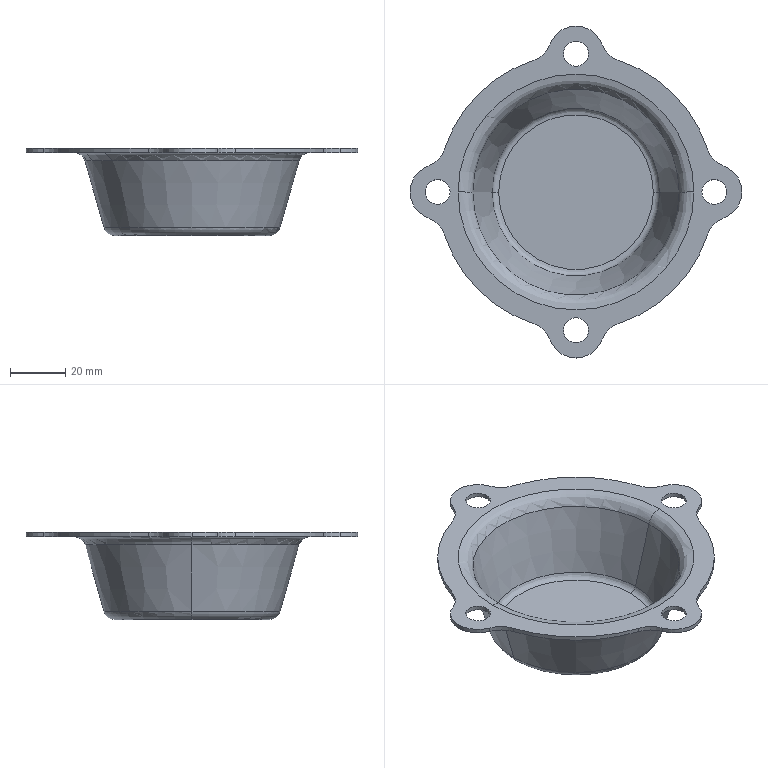Part | SolidWorks | features Boss 1, Extrusion 1, Fillet 1, RefAxis 1, Shell 1 | 1 solid | 41 faces | box 120 x 120 x 31.5 mm | volume 19269 mm3 | cylinder 25 | torus 8 | cone 4 | plane 4 | commonest cylinder face diameters 20 x13 9 x8 100 x4
STEP:
#1=CARTESIAN_POINT('',(42.584,0.,1.5));
#2=VERTEX_POINT('',#1);
#3=CARTESIAN_POINT('',(-42.584,0.,1.5));
#4=VERTEX_POINT('',#3);
#5=CARTESIAN_POINT('',(0.,0.,1.5));
#6=DIRECTION('',(0.,0.,1.));
#7=DIRECTION('',(1.,0.,0.));
#8=AXIS2_PLACEMENT_3D('',#5,#6,#7);
#9=CIRCLE('',#8,42.584);
#10=EDGE_CURVE('',#2,#4,#9,.T.);
#11=ORIENTED_EDGE('',*,*,#10,.T.);
#12=CARTESIAN_POINT('',(-37.297,0.,-2.484));
#13=VERTEX_POINT('',#12);
#14=CARTESIAN_POINT('',(-42.584,0.,-4.));
#15=DIRECTION('',(0.,1.,0.));
#16=DIRECTION('',(-1.,0.,0.));
#17=AXIS2_PLACEMENT_3D('',#14,#15,#16);
#18=CIRCLE('',#17,5.5);
#19=EDGE_CURVE('',#4,#13,#18,.T.);
#20=ORIENTED_EDGE('',*,*,#19,.T.);
#21=CARTESIAN_POINT('',(37.297,0.,-2.484));
#22=VERTEX_POINT('',#21);
#23=CARTESIAN_POINT('',(0.,0.,-2.484));
#24=DIRECTION('',(0.,0.,-1.));
#25=DIRECTION('',(1.,0.,0.));
#26=AXIS2_PLACEMENT_3D('',#23,#24,#25);
#27=CIRCLE('',#26,37.297);
#28=EDGE_CURVE('',#13,#22,#27,.T.);
#29=ORIENTED_EDGE('',*,*,#28,.T.);
#30=CARTESIAN_POINT('',(42.584,0.,-4.));
#31=DIRECTION('',(0.,-1.,0.));
#32=DIRECTION('',(0.,0.,-1.));
#33=AXIS2_PLACEMENT_3D('',#30,#31,#32);
#34=CIRCLE('',#33,5.5);
#35=EDGE_CURVE('',#2,#22,#34,.T.);
#36=ORIENTED_EDGE('',*,*,#35,.F.);
#37=EDGE_LOOP('',(#11,#20,#29,#36));
#38=FACE_OUTER_BOUND('',#37,.T.);
#39=CARTESIAN_POINT('',(0.,0.,-4.));
#40=DIRECTION('',(0.,0.,1.));
#41=DIRECTION('',(1.,0.,0.));
#42=AXIS2_PLACEMENT_3D('',#39,#40,#41);
#43=TOROIDAL_SURFACE('',#42,42.584,5.5);
#44=ADVANCED_FACE('',(#38),#43,.T.);
#45=CARTESIAN_POINT('',(27.953,0.,-28.5));
#46=VERTEX_POINT('',#45);
#47=CARTESIAN_POINT('',(-27.953,0.,-28.5));
#48=VERTEX_POINT('',#47);
#49=CARTESIAN_POINT('',(0.,0.,-28.5));
#50=DIRECTION('',(0.,0.,-1.));
#51=DIRECTION('',(1.,0.,0.));
#52=AXIS2_PLACEMENT_3D('',#49,#50,#51);
#53=CIRCLE('',#52,27.953);
#54=EDGE_CURVE('',#46,#48,#53,.T.);
#55=ORIENTED_EDGE('',*,*,#54,.T.);
#56=CARTESIAN_POINT('',(-30.356,0.,-26.689));
#57=VERTEX_POINT('',#56);
#58=CARTESIAN_POINT('',(-27.953,0.,-26.));
#59=DIRECTION('',(0.,1.,0.));
#60=DIRECTION('',(-1.,0.,0.));
#61=AXIS2_PLACEMENT_3D('',#58,#59,#60);
#62=CIRCLE('',#61,2.5);
#63=EDGE_CURVE('',#48,#57,#62,.T.);
#64=ORIENTED_EDGE('',*,*,#63,.T.);
#65=CARTESIAN_POINT('',(30.356,0.,-26.689));
#66=VERTEX_POINT('',#65);
#67=CARTESIAN_POINT('',(0.,0.,-26.689));
#68=DIRECTION('',(0.,0.,1.));
#69=DIRECTION('',(1.,0.,0.));
#70=AXIS2_PLACEMENT_3D('',#67,#68,#69);
#71=CIRCLE('',#70,30.356);
#72=EDGE_CURVE('',#57,#66,#71,.T.);
#73=ORIENTED_EDGE('',*,*,#72,.T.);
#74=CARTESIAN_POINT('',(27.953,0.,-26.));
#75=DIRECTION('',(0.,-1.,0.));
#76=DIRECTION('',(0.,0.,-1.));
#77=AXIS2_PLACEMENT_3D('',#74,#75,#76);
#78=CIRCLE('',#77,2.5);
#79=EDGE_CURVE('',#46,#66,#78,.T.);
#80=ORIENTED_EDGE('',*,*,#79,.F.);
#81=EDGE_LOOP('',(#55,#64,#73,#80));
#82=FACE_OUTER_BOUND('',#81,.T.);
#83=CARTESIAN_POINT('',(0.,0.,-26.));
#84=DIRECTION('',(0.,0.,1.));
#85=DIRECTION('',(1.,0.,0.));
#86=AXIS2_PLACEMENT_3D('',#83,#84,#85);
#87=TOROIDAL_SURFACE('',#86,27.953,2.5);
#88=ADVANCED_FACE('',(#82),#87,.F.);
#89=ORIENTED_EDGE('',*,*,#72,.F.);
#90=CARTESIAN_POINT('',(-38.558,0.,1.913));
#91=DIRECTION('',(-0.2756,0.,0.9613));
#92=VECTOR('',#91,1000.);
#93=LINE('',#90,#92);
#94=EDGE_CURVE('',#57,#13,#93,.T.);
#95=ORIENTED_EDGE('',*,*,#94,.T.);
#96=CARTESIAN_POINT('',(0.,0.,-2.484));
#97=DIRECTION('',(0.,0.,-1.));
#98=DIRECTION('',(1.,0.,0.));
#99=AXIS2_PLACEMENT_3D('',#96,#97,#98);
#100=CIRCLE('',#99,37.297);
#101=EDGE_CURVE('',#22,#13,#100,.T.);
#102=ORIENTED_EDGE('',*,*,#101,.F.);
#103=CARTESIAN_POINT('',(38.558,0.,1.913));
#104=DIRECTION('',(0.2756,0.,0.9613));
#105=VECTOR('',#104,1000.);
#106=LINE('',#103,#105);
#107=EDGE_CURVE('',#66,#22,#106,.T.);
#108=ORIENTED_EDGE('',*,*,#107,.F.);
#109=EDGE_LOOP('',(#89,#95,#102,#108));
#110=FACE_OUTER_BOUND('',#109,.T.);
#111=CARTESIAN_POINT('',(0.,0.,1.913));
#112=DIRECTION('',(0.,0.,1.));
#113=DIRECTION('',(1.,0.,0.));
#114=AXIS2_PLACEMENT_3D('',#111,#112,#113);
#115=CONICAL_SURFACE('',#114,38.558,0.2793);
#116=ADVANCED_FACE('',(#110),#115,.F.);
#117=CARTESIAN_POINT('',(-42.584,0.,0.));
#118=VERTEX_POINT('',#117);
#119=CARTESIAN_POINT('',(42.584,0.,0.));
#120=VERTEX_POINT('',#119);
#121=CARTESIAN_POINT('',(0.,0.,0.));
#122=DIRECTION('',(0.,0.,1.));
#123=DIRECTION('',(1.,0.,0.));
#124=AXIS2_PLACEMENT_3D('',#121,#122,#123);
#125=CIRCLE('',#124,42.584);
#126=EDGE_CURVE('',#118,#120,#125,.T.);
#127=ORIENTED_EDGE('',*,*,#126,.F.);
#128=CARTESIAN_POINT('',(-38.739,0.,-2.897));
#129=VERTEX_POINT('',#128);
#130=CARTESIAN_POINT('',(-42.584,0.,-4.));
#131=DIRECTION('',(0.,1.,0.));
#132=DIRECTION('',(-1.,0.,0.));
#133=AXIS2_PLACEMENT_3D('',#130,#131,#132);
#134=CIRCLE('',#133,4.);
#135=EDGE_CURVE('',#118,#129,#134,.T.);
#136=ORIENTED_EDGE('',*,*,#135,.T.);
#137=CARTESIAN_POINT('',(38.739,0.,-2.897));
#138=VERTEX_POINT('',#137);
#139=CARTESIAN_POINT('',(0.,0.,-2.897));
#140=DIRECTION('',(0.,0.,-1.));
#141=DIRECTION('',(-1.,0.,0.));
#142=AXIS2_PLACEMENT_3D('',#139,#140,#141);
#143=CIRCLE('',#142,38.739);
#144=EDGE_CURVE('',#138,#129,#143,.T.);
#145=ORIENTED_EDGE('',*,*,#144,.F.);
#146=CARTESIAN_POINT('',(42.584,0.,-4.));
#147=DIRECTION('',(0.,-1.,0.));
#148=DIRECTION('',(0.,0.,-1.));
#149=AXIS2_PLACEMENT_3D('',#146,#147,#148);
#150=CIRCLE('',#149,4.);
#151=EDGE_CURVE('',#120,#138,#150,.T.);
#152=ORIENTED_EDGE('',*,*,#151,.F.);
#153=EDGE_LOOP('',(#127,#136,#145,#152));
#154=FACE_OUTER_BOUND('',#153,.T.);
#155=CARTESIAN_POINT('',(0.,0.,-4.));
#156=DIRECTION('',(0.,0.,1.));
#157=DIRECTION('',(1.,0.,0.));
#158=AXIS2_PLACEMENT_3D('',#155,#156,#157);
#159=TOROIDAL_SURFACE('',#158,42.584,4.);
#160=ADVANCED_FACE('',(#154),#159,.F.);
#161=CARTESIAN_POINT('',(-27.953,0.,-30.));
#162=VERTEX_POINT('',#161);
#163=CARTESIAN_POINT('',(27.953,0.,-30.));
#164=VERTEX_POINT('',#163);
#165=CARTESIAN_POINT('',(0.,0.,-30.));
#166=DIRECTION('',(0.,0.,-1.));
#167=DIRECTION('',(1.,0.,0.));
#168=AXIS2_PLACEMENT_3D('',#165,#166,#167);
#169=CIRCLE('',#168,27.953);
#170=EDGE_CURVE('',#162,#164,#169,.T.);
#171=ORIENTED_EDGE('',*,*,#170,.F.);
#172=CARTESIAN_POINT('',(-31.798,0.,-27.103));
#173=VERTEX_POINT('',#172);
#174=CARTESIAN_POINT('',(-27.953,0.,-26.));
#175=DIRECTION('',(0.,1.,0.));
#176=DIRECTION('',(-1.,0.,0.));
#177=AXIS2_PLACEMENT_3D('',#174,#175,#176);
#178=CIRCLE('',#177,4.);
#179=EDGE_CURVE('',#162,#173,#178,.T.);
#180=ORIENTED_EDGE('',*,*,#179,.T.);
#181=CARTESIAN_POINT('',(31.798,0.,-27.103));
#182=VERTEX_POINT('',#181);
#183=CARTESIAN_POINT('',(0.,0.,-27.103));
#184=DIRECTION('',(0.,0.,1.));
#185=DIRECTION('',(1.,0.,0.));
#186=AXIS2_PLACEMENT_3D('',#183,#184,#185);
#187=CIRCLE('',#186,31.798);
#188=EDGE_CURVE('',#182,#173,#187,.T.);
#189=ORIENTED_EDGE('',*,*,#188,.F.);
#190=CARTESIAN_POINT('',(27.953,0.,-26.));
#191=DIRECTION('',(0.,-1.,0.));
#192=DIRECTION('',(0.,0.,-1.));
#193=AXIS2_PLACEMENT_3D('',#190,#191,#192);
#194=CIRCLE('',#193,4.);
#195=EDGE_CURVE('',#164,#182,#194,.T.);
#196=ORIENTED_EDGE('',*,*,#195,.F.);
#197=EDGE_LOOP('',(#171,#180,#189,#196));
#198=FACE_OUTER_BOUND('',#197,.T.);
#199=CARTESIAN_POINT('',(0.,0.,-26.));
#200=DIRECTION('',(0.,0.,1.));
#201=DIRECTION('',(1.,0.,0.));
#202=AXIS2_PLACEMENT_3D('',#199,#200,#201);
#203=TOROIDAL_SURFACE('',#202,27.953,4.);
#204=ADVANCED_FACE('',(#198),#203,.T.);
#205=ORIENTED_EDGE('',*,*,#188,.T.);
#206=CARTESIAN_POINT('',(-40.,0.,1.5));
#207=DIRECTION('',(-0.2756,0.,0.9613));
#208=VECTOR('',#207,1000.);
#209=LINE('',#206,#208);
#210=EDGE_CURVE('',#173,#129,#209,.T.);
#211=ORIENTED_EDGE('',*,*,#210,.T.);
#212=CARTESIAN_POINT('',(0.,0.,-2.897));
#213=DIRECTION('',(0.,0.,-1.));
#214=DIRECTION('',(-1.,0.,0.));
#215=AXIS2_PLACEMENT_3D('',#212,#213,#214);
#216=CIRCLE('',#215,38.739);
#217=EDGE_CURVE('',#129,#138,#216,.T.);
#218=ORIENTED_EDGE('',*,*,#217,.T.);
#219=CARTESIAN_POINT('',(40.,0.,1.5));
#220=DIRECTION('',(0.2756,0.,0.9613));
#221=VECTOR('',#220,1000.);
#222=LINE('',#219,#221);
#223=EDGE_CURVE('',#182,#138,#222,.T.);
#224=ORIENTED_EDGE('',*,*,#223,.F.);
#225=EDGE_LOOP('',(#205,#211,#218,#224));
#226=FACE_OUTER_BOUND('',#225,.T.);
#227=CARTESIAN_POINT('',(0.,0.,1.5));
#228=DIRECTION('',(0.,0.,1.));
#229=DIRECTION('',(1.,0.,0.));
#230=AXIS2_PLACEMENT_3D('',#227,#228,#229);
#231=CONICAL_SURFACE('',#230,40.,0.2793);
#232=ADVANCED_FACE('',(#226),#231,.T.);
#233=CARTESIAN_POINT('',(45.5,0.,1.5));
#234=VERTEX_POINT('',#233);
#235=CARTESIAN_POINT('',(54.5,0.,1.5));
#236=VERTEX_POINT('',#235);
#237=CARTESIAN_POINT('',(50.,0.,1.5));
#238=DIRECTION('',(0.,0.,1.));
#239=DIRECTION('',(1.,0.,0.));
#240=AXIS2_PLACEMENT_3D('',#237,#238,#239);
#241=CIRCLE('',#240,4.5);
#242=EDGE_CURVE('',#234,#236,#241,.T.);
#243=ORIENTED_EDGE('',*,*,#242,.T.);
#244=CARTESIAN_POINT('',(54.5,0.,0.));
#245=VERTEX_POINT('',#244);
#246=CARTESIAN_POINT('',(54.5,0.,1.5));
#247=DIRECTION('',(0.,0.,-1.));
#248=VECTOR('',#247,1000.);
#249=LINE('',#246,#248);
#250=EDGE_CURVE('',#236,#245,#249,.T.);
#251=ORIENTED_EDGE('',*,*,#250,.T.);
#252=CARTESIAN_POINT('',(45.5,0.,0.));
#253=VERTEX_POINT('',#252);
#254=CARTESIAN_POINT('',(50.,0.,0.));
#255=DIRECTION('',(0.,0.,1.));
#256=DIRECTION('',(1.,0.,0.));
#257=AXIS2_PLACEMENT_3D('',#254,#255,#256);
#258=CIRCLE('',#257,4.5);
#259=EDGE_CURVE('',#253,#245,#258,.T.);
#260=ORIENTED_EDGE('',*,*,#259,.F.);
#261=CARTESIAN_POINT('',(45.5,0.,1.5));
#262=DIRECTION('',(0.,0.,-1.));
#263=VECTOR('',#262,1000.);
#264=LINE('',#261,#263);
#265=EDGE_CURVE('',#234,#253,#264,.T.);
#266=ORIENTED_EDGE('',*,*,#265,.F.);
#267=EDGE_LOOP('',(#243,#251,#260,#266));
#268=FACE_OUTER_BOUND('',#267,.T.);
#269=CARTESIAN_POINT('',(50.,0.,1.5));
#270=DIRECTION('',(0.,0.,-1.));
#271=DIRECTION('',(-1.,0.,0.));
#272=AXIS2_PLACEMENT_3D('',#269,#270,#271);
#273=CYLINDRICAL_SURFACE('',#272,4.5);
#274=ADVANCED_FACE('',(#268),#273,.F.);
#275=CARTESIAN_POINT('',(-4.5,-50.,1.5));
#276=VERTEX_POINT('',#275);
#277=CARTESIAN_POINT('',(4.5,-50.,1.5));
#278=VERTEX_POINT('',#277);
#279=CARTESIAN_POINT('',(0.,-50.,1.5));
#280=DIRECTION('',(0.,0.,1.));
#281=DIRECTION('',(1.,0.,0.));
#282=AXIS2_PLACEMENT_3D('',#279,#280,#281);
#283=CIRCLE('',#282,4.5);
#284=EDGE_CURVE('',#276,#278,#283,.T.);
#285=ORIENTED_EDGE('',*,*,#284,.T.);
#286=CARTESIAN_POINT('',(4.5,-50.,0.));
#287=VERTEX_POINT('',#286);
#288=CARTESIAN_POINT('',(4.5,-50.,1.5));
#289=DIRECTION('',(0.,0.,-1.));
#290=VECTOR('',#289,1000.);
#291=LINE('',#288,#290);
#292=EDGE_CURVE('',#278,#287,#291,.T.);
#293=ORIENTED_EDGE('',*,*,#292,.T.);
#294=CARTESIAN_POINT('',(-4.5,-50.,0.));
#295=VERTEX_POINT('',#294);
#296=CARTESIAN_POINT('',(0.,-50.,0.));
#297=DIRECTION('',(0.,0.,1.));
#298=DIRECTION('',(1.,0.,0.));
#299=AXIS2_PLACEMENT_3D('',#296,#297,#298);
#300=CIRCLE('',#299,4.5);
#301=EDGE_CURVE('',#295,#287,#300,.T.);
#302=ORIENTED_EDGE('',*,*,#301,.F.);
#303=CARTESIAN_POINT('',(-4.5,-50.,1.5));
#304=DIRECTION('',(0.,0.,-1.));
#305=VECTOR('',#304,1000.);
#306=LINE('',#303,#305);
#307=EDGE_CURVE('',#276,#295,#306,.T.);
#308=ORIENTED_EDGE('',*,*,#307,.F.);
#309=EDGE_LOOP('',(#285,#293,#302,#308));
#310=FACE_OUTER_BOUND('',#309,.T.);
#311=CARTESIAN_POINT('',(0.,-50.,1.5));
#312=DIRECTION('',(0.,0.,-1.));
#313=DIRECTION('',(-1.,0.,0.));
#314=AXIS2_PLACEMENT_3D('',#311,#312,#313);
#315=CYLINDRICAL_SURFACE('',#314,4.5);
#316=ADVANCED_FACE('',(#310),#315,.F.);
#317=CARTESIAN_POINT('',(-54.5,0.,1.5));
#318=VERTEX_POINT('',#317);
#319=CARTESIAN_POINT('',(-45.5,0.,1.5));
#320=VERTEX_POINT('',#319);
#321=CARTESIAN_POINT('',(-50.,0.,1.5));
#322=DIRECTION('',(0.,0.,1.));
#323=DIRECTION('',(1.,0.,0.));
#324=AXIS2_PLACEMENT_3D('',#321,#322,#323);
#325=CIRCLE('',#324,4.5);
#326=EDGE_CURVE('',#318,#320,#325,.T.);
#327=ORIENTED_EDGE('',*,*,#326,.T.);
#328=CARTESIAN_POINT('',(-45.5,0.,0.));
#329=VERTEX_POINT('',#328);
#330=CARTESIAN_POINT('',(-45.5,0.,1.5));
#331=DIRECTION('',(0.,0.,-1.));
#332=VECTOR('',#331,1000.);
#333=LINE('',#330,#332);
#334=EDGE_CURVE('',#320,#329,#333,.T.);
#335=ORIENTED_EDGE('',*,*,#334,.T.);
#336=CARTESIAN_POINT('',(-54.5,0.,0.));
#337=VERTEX_POINT('',#336);
#338=CARTESIAN_POINT('',(-50.,0.,0.));
#339=DIRECTION('',(0.,0.,1.));
#340=DIRECTION('',(1.,0.,0.));
#341=AXIS2_PLACEMENT_3D('',#338,#339,#340);
#342=CIRCLE('',#341,4.5);
#343=EDGE_CURVE('',#337,#329,#342,.T.);
#344=ORIENTED_EDGE('',*,*,#343,.F.);
#345=CARTESIAN_POINT('',(-54.5,0.,1.5));
#346=DIRECTION('',(0.,0.,-1.));
#347=VECTOR('',#346,1000.);
#348=LINE('',#345,#347);
#349=EDGE_CURVE('',#318,#337,#348,.T.);
#350=ORIENTED_EDGE('',*,*,#349,.F.);
#351=EDGE_LOOP('',(#327,#335,#344,#350));
#352=FACE_OUTER_BOUND('',#351,.T.);
#353=CARTESIAN_POINT('',(-50.,0.,1.5));
#354=DIRECTION('',(0.,0.,-1.));
#355=DIRECTION('',(-1.,0.,0.));
#356=AXIS2_PLACEMENT_3D('',#353,#354,#355);
#357=CYLINDRICAL_SURFACE('',#356,4.5);
#358=ADVANCED_FACE('',(#352),#357,.F.);
#359=CARTESIAN_POINT('',(-4.5,50.,1.5));
#360=VERTEX_POINT('',#359);
#361=CARTESIAN_POINT('',(4.5,50.,1.5));
#362=VERTEX_POINT('',#361);
#363=CARTESIAN_POINT('',(0.,50.,1.5));
#364=DIRECTION('',(0.,0.,1.));
#365=DIRECTION('',(1.,0.,0.));
#366=AXIS2_PLACEMENT_3D('',#363,#364,#365);
#367=CIRCLE('',#366,4.5);
#368=EDGE_CURVE('',#360,#362,#367,.T.);
#369=ORIENTED_EDGE('',*,*,#368,.T.);
#370=CARTESIAN_POINT('',(4.5,50.,0.));
#371=VERTEX_POINT('',#370);
#372=CARTESIAN_POINT('',(4.5,50.,1.5));
#373=DIRECTION('',(0.,0.,-1.));
#374=VECTOR('',#373,1000.);
#375=LINE('',#372,#374);
#376=EDGE_CURVE('',#362,#371,#375,.T.);
#377=ORIENTED_EDGE('',*,*,#376,.T.);
#378=CARTESIAN_POINT('',(-4.5,50.,0.));
#379=VERTEX_POINT('',#378);
#380=CARTESIAN_POINT('',(0.,50.,0.));
#381=DIRECTION('',(0.,0.,1.));
#382=DIRECTION('',(1.,0.,0.));
#383=AXIS2_PLACEMENT_3D('',#380,#381,#382);
#384=CIRCLE('',#383,4.5);
#385=EDGE_CURVE('',#379,#371,#384,.T.);
#386=ORIENTED_EDGE('',*,*,#385,.F.);
#387=CARTESIAN_POINT('',(-4.5,50.,1.5));
#388=DIRECTION('',(0.,0.,-1.));
#389=VECTOR('',#388,1000.);
#390=LINE('',#387,#389);
#391=EDGE_CURVE('',#360,#379,#390,.T.);
#392=ORIENTED_EDGE('',*,*,#391,.F.);
#393=EDGE_LOOP('',(#369,#377,#386,#392));
#394=FACE_OUTER_BOUND('',#393,.T.);
#395=CARTESIAN_POINT('',(0.,50.,1.5));
#396=DIRECTION('',(0.,0.,-1.));
#397=DIRECTION('',(-1.,0.,0.));
#398=AXIS2_PLACEMENT_3D('',#395,#396,#397);
#399=CYLINDRICAL_SURFACE('',#398,4.5);
#400=ADVANCED_FACE('',(#394),#399,.F.);
#401=CARTESIAN_POINT('',(-60.,0.,1.5));
#402=VERTEX_POINT('',#401);
#403=CARTESIAN_POINT('',(-53.5,-9.367,1.5));
#404=VERTEX_POINT('',#403);
#405=CARTESIAN_POINT('',(-50.,0.,1.5));
#406=DIRECTION('',(0.,0.,1.));
#407=DIRECTION('',(1.,0.,0.));
#408=AXIS2_PLACEMENT_3D('',#405,#406,#407);
#409=CIRCLE('',#408,10.);
#410=EDGE_CURVE('',#402,#404,#409,.T.);
#411=ORIENTED_EDGE('',*,*,#410,.F.);
#412=CARTESIAN_POINT('',(-60.,0.,0.));
#413=VERTEX_POINT('',#412);
#414=CARTESIAN_POINT('',(-60.,0.,1.5));
#415=DIRECTION('',(0.,0.,-1.));
#416=VECTOR('',#415,1000.);
#417=LINE('',#414,#416);
#418=EDGE_CURVE('',#402,#413,#417,.T.);
#419=ORIENTED_EDGE('',*,*,#418,.T.);
#420=CARTESIAN_POINT('',(-53.5,-9.367,0.));
#421=VERTEX_POINT('',#420);
#422=CARTESIAN_POINT('',(-50.,0.,0.));
#423=DIRECTION('',(0.,0.,1.));
#424=DIRECTION('',(1.,0.,0.));
#425=AXIS2_PLACEMENT_3D('',#422,#423,#424);
#426=CIRCLE('',#425,10.);
#427=EDGE_CURVE('',#413,#421,#426,.T.);
#428=ORIENTED_EDGE('',*,*,#427,.T.);
#429=CARTESIAN_POINT('',(-53.5,-9.367,1.5));
#430=DIRECTION('',(0.,0.,-1.));
#431=VECTOR('',#430,1000.);
#432=LINE('',#429,#431);
#433=EDGE_CURVE('',#404,#421,#432,.T.);
#434=ORIENTED_EDGE('',*,*,#433,.F.);
#435=EDGE_LOOP('',(#411,#419,#428,#434));
#436=FACE_OUTER_BOUND('',#435,.T.);
#437=CARTESIAN_POINT('',(-50.,0.,1.5));
#438=DIRECTION('',(0.,0.,-1.));
#439=DIRECTION('',(-1.,0.,0.));
#440=AXIS2_PLACEMENT_3D('',#437,#438,#439);
#441=CYLINDRICAL_SURFACE('',#440,10.);
#442=ADVANCED_FACE('',(#436),#441,.T.);
#443=ORIENTED_EDGE('',*,*,#10,.F.);
#444=CARTESIAN_POINT('',(0.,0.,1.5));
#445=DIRECTION('',(0.,0.,1.));
#446=DIRECTION('',(1.,0.,0.));
#447=AXIS2_PLACEMENT_3D('',#444,#445,#446);
#448=CIRCLE('',#447,42.584);
#449=EDGE_CURVE('',#4,#2,#448,.T.);
#450=ORIENTED_EDGE('',*,*,#449,.F.);
#451=EDGE_LOOP('',(#443,#450));
#452=FACE_BOUND('',#451,.T.);
#453=ORIENTED_EDGE('',*,*,#284,.F.);
#454=CARTESIAN_POINT('',(0.,-50.,1.5));
#455=DIRECTION('',(0.,0.,1.));
#456=DIRECTION('',(1.,0.,0.));
#457=AXIS2_PLACEMENT_3D('',#454,#455,#456);
#458=CIRCLE('',#457,4.5);
#459=EDGE_CURVE('',#278,#276,#458,.T.);
#460=ORIENTED_EDGE('',*,*,#459,.F.);
#461=EDGE_LOOP('',(#453,#460));
#462=FACE_BOUND('',#461,.T.);
#463=ORIENTED_EDGE('',*,*,#368,.F.);
#464=CARTESIAN_POINT('',(0.,50.,1.5));
#465=DIRECTION('',(0.,0.,1.));
#466=DIRECTION('',(1.,0.,0.));
#467=AXIS2_PLACEMENT_3D('',#464,#465,#466);
#468=CIRCLE('',#467,4.5);
#469=EDGE_CURVE('',#362,#360,#468,.T.);
#470=ORIENTED_EDGE('',*,*,#469,.F.);
#471=EDGE_LOOP('',(#463,#470));
#472=FACE_BOUND('',#471,.T.);
#473=CARTESIAN_POINT('',(-9.367,53.5,1.5));
#474=VERTEX_POINT('',#473);
#475=CARTESIAN_POINT('',(-15.612,47.5,1.5));
#476=VERTEX_POINT('',#475);
#477=CARTESIAN_POINT('',(-18.735,57.,1.5));
#478=DIRECTION('',(0.,0.,-1.));
#479=DIRECTION('',(1.,0.,0.));
#480=AXIS2_PLACEMENT_3D('',#477,#478,#479);
#481=CIRCLE('',#480,10.);
#482=EDGE_CURVE('',#474,#476,#481,.T.);
#483=ORIENTED_EDGE('',*,*,#482,.T.);
#484=CARTESIAN_POINT('',(-47.5,15.612,1.5));
#485=VERTEX_POINT('',#484);
#486=CARTESIAN_POINT('',(0.,0.,1.5));
#487=DIRECTION('',(0.,0.,1.));
#488=DIRECTION('',(1.,0.,0.));
#489=AXIS2_PLACEMENT_3D('',#486,#487,#488);
#490=CIRCLE('',#489,50.);
#491=EDGE_CURVE('',#476,#485,#490,.T.);
#492=ORIENTED_EDGE('',*,*,#491,.T.);
#493=CARTESIAN_POINT('',(-53.5,9.367,1.5));
#494=VERTEX_POINT('',#493);
#495=CARTESIAN_POINT('',(-57.,18.735,1.5));
#496=DIRECTION('',(0.,0.,-1.));
#497=DIRECTION('',(-1.,0.,0.));
#498=AXIS2_PLACEMENT_3D('',#495,#496,#497);
#499=CIRCLE('',#498,10.);
#500=EDGE_CURVE('',#485,#494,#499,.T.);
#501=ORIENTED_EDGE('',*,*,#500,.T.);
#502=CARTESIAN_POINT('',(-50.,0.,1.5));
#503=DIRECTION('',(0.,0.,1.));
#504=DIRECTION('',(1.,0.,0.));
#505=AXIS2_PLACEMENT_3D('',#502,#503,#504);
#506=CIRCLE('',#505,10.);
#507=EDGE_CURVE('',#494,#402,#506,.T.);
#508=ORIENTED_EDGE('',*,*,#507,.T.);
#509=ORIENTED_EDGE('',*,*,#410,.T.);
#510=CARTESIAN_POINT('',(-47.5,-15.612,1.5));
#511=VERTEX_POINT('',#510);
#512=CARTESIAN_POINT('',(-57.,-18.735,1.5));
#513=DIRECTION('',(0.,0.,-1.));
#514=DIRECTION('',(-1.,0.,0.));
#515=AXIS2_PLACEMENT_3D('',#512,#513,#514);
#516=CIRCLE('',#515,10.);
#517=EDGE_CURVE('',#404,#511,#516,.T.);
#518=ORIENTED_EDGE('',*,*,#517,.T.);
#519=CARTESIAN_POINT('',(-15.612,-47.5,1.5));
#520=VERTEX_POINT('',#519);
#521=CARTESIAN_POINT('',(0.,0.,1.5));
#522=DIRECTION('',(0.,0.,1.));
#523=DIRECTION('',(1.,0.,0.));
#524=AXIS2_PLACEMENT_3D('',#521,#522,#523);
#525=CIRCLE('',#524,50.);
#526=EDGE_CURVE('',#511,#520,#525,.T.);
#527=ORIENTED_EDGE('',*,*,#526,.T.);
#528=CARTESIAN_POINT('',(-9.367,-53.5,1.5));
#529=VERTEX_POINT('',#528);
#530=CARTESIAN_POINT('',(-18.735,-57.,1.5));
#531=DIRECTION('',(0.,0.,-1.));
#532=DIRECTION('',(-1.,0.,0.));
#533=AXIS2_PLACEMENT_3D('',#530,#531,#532);
#534=CIRCLE('',#533,10.);
#535=EDGE_CURVE('',#520,#529,#534,.T.);
#536=ORIENTED_EDGE('',*,*,#535,.T.);
#537=CARTESIAN_POINT('',(9.367,-53.5,1.5));
#538=VERTEX_POINT('',#537);
#539=CARTESIAN_POINT('',(0.,-50.,1.5));
#540=DIRECTION('',(0.,0.,1.));
#541=DIRECTION('',(1.,0.,0.));
#542=AXIS2_PLACEMENT_3D('',#539,#540,#541);
#543=CIRCLE('',#542,10.);
#544=EDGE_CURVE('',#529,#538,#543,.T.);
#545=ORIENTED_EDGE('',*,*,#544,.T.);
#546=CARTESIAN_POINT('',(15.612,-47.5,1.5));
#547=VERTEX_POINT('',#546);
#548=CARTESIAN_POINT('',(18.735,-57.,1.5));
#549=DIRECTION('',(0.,0.,-1.));
#550=DIRECTION('',(-1.,0.,0.));
#551=AXIS2_PLACEMENT_3D('',#548,#549,#550);
#552=CIRCLE('',#551,10.);
#553=EDGE_CURVE('',#538,#547,#552,.T.);
#554=ORIENTED_EDGE('',*,*,#553,.T.);
#555=CARTESIAN_POINT('',(47.5,-15.612,1.5));
#556=VERTEX_POINT('',#555);
#557=CARTESIAN_POINT('',(0.,0.,1.5));
#558=DIRECTION('',(0.,0.,1.));
#559=DIRECTION('',(1.,0.,0.));
#560=AXIS2_PLACEMENT_3D('',#557,#558,#559);
#561=CIRCLE('',#560,50.);
#562=EDGE_CURVE('',#547,#556,#561,.T.);
#563=ORIENTED_EDGE('',*,*,#562,.T.);
#564=CARTESIAN_POINT('',(53.5,-9.367,1.5));
#565=VERTEX_POINT('',#564);
#566=CARTESIAN_POINT('',(57.,-18.735,1.5));
#567=DIRECTION('',(0.,0.,-1.));
#568=DIRECTION('',(-1.,0.,0.));
#569=AXIS2_PLACEMENT_3D('',#566,#567,#568);
#570=CIRCLE('',#569,10.);
#571=EDGE_CURVE('',#556,#565,#570,.T.);
#572=ORIENTED_EDGE('',*,*,#571,.T.);
#573=CARTESIAN_POINT('',(53.5,9.367,1.5));
#574=VERTEX_POINT('',#573);
#575=CARTESIAN_POINT('',(50.,0.,1.5));
#576=DIRECTION('',(0.,0.,1.));
#577=DIRECTION('',(1.,0.,0.));
#578=AXIS2_PLACEMENT_3D('',#575,#576,#577);
#579=CIRCLE('',#578,10.);
#580=EDGE_CURVE('',#565,#574,#579,.T.);
#581=ORIENTED_EDGE('',*,*,#580,.T.);
#582=CARTESIAN_POINT('',(47.5,15.612,1.5));
#583=VERTEX_POINT('',#582);
#584=CARTESIAN_POINT('',(57.,18.735,1.5));
#585=DIRECTION('',(0.,0.,-1.));
#586=DIRECTION('',(-1.,0.,0.));
#587=AXIS2_PLACEMENT_3D('',#584,#585,#586);
#588=CIRCLE('',#587,10.);
#589=EDGE_CURVE('',#574,#583,#588,.T.);
#590=ORIENTED_EDGE('',*,*,#589,.T.);
#591=CARTESIAN_POINT('',(15.612,47.5,1.5));
#592=VERTEX_POINT('',#591);
#593=CARTESIAN_POINT('',(0.,0.,1.5));
#594=DIRECTION('',(0.,0.,1.));
#595=DIRECTION('',(1.,0.,0.));
#596=AXIS2_PLACEMENT_3D('',#593,#594,#595);
#597=CIRCLE('',#596,50.);
#598=EDGE_CURVE('',#583,#592,#597,.T.);
#599=ORIENTED_EDGE('',*,*,#598,.T.);
#600=CARTESIAN_POINT('',(9.367,53.5,1.5));
#601=VERTEX_POINT('',#600);
#602=CARTESIAN_POINT('',(18.735,57.,1.5));
#603=DIRECTION('',(0.,0.,-1.));
#604=DIRECTION('',(-1.,0.,0.));
#605=AXIS2_PLACEMENT_3D('',#602,#603,#604);
#606=CIRCLE('',#605,10.);
#607=EDGE_CURVE('',#592,#601,#606,.T.);
#608=ORIENTED_EDGE('',*,*,#607,.T.);
#609=CARTESIAN_POINT('',(0.,50.,1.5));
#610=DIRECTION('',(0.,0.,1.));
#611=DIRECTION('',(1.,0.,0.));
#612=AXIS2_PLACEMENT_3D('',#609,#610,#611);
#613=CIRCLE('',#612,10.);
#614=EDGE_CURVE('',#601,#474,#613,.T.);
#615=ORIENTED_EDGE('',*,*,#614,.T.);
#616=EDGE_LOOP('',(#483,#492,#501,#508,#509,#518,#527,#536,#545,#554,#563,#572,#581,#590,#599,#608,#615));
#617=FACE_OUTER_BOUND('',#616,.T.);
#618=ORIENTED_EDGE('',*,*,#326,.F.);
#619=CARTESIAN_POINT('',(-50.,0.,1.5));
#620=DIRECTION('',(0.,0.,1.));
#621=DIRECTION('',(1.,0.,0.));
#622=AXIS2_PLACEMENT_3D('',#619,#620,#621);
#623=CIRCLE('',#622,4.5);
#624=EDGE_CURVE('',#320,#318,#623,.T.);
#625=ORIENTED_EDGE('',*,*,#624,.F.);
#626=EDGE_LOOP('',(#618,#625));
#627=FACE_BOUND('',#626,.T.);
#628=ORIENTED_EDGE('',*,*,#242,.F.);
#629=CARTESIAN_POINT('',(50.,0.,1.5));
#630=DIRECTION('',(0.,0.,1.));
#631=DIRECTION('',(1.,0.,0.));
#632=AXIS2_PLACEMENT_3D('',#629,#630,#631);
#633=CIRCLE('',#632,4.5);
#634=EDGE_CURVE('',#236,#234,#633,.T.);
#635=ORIENTED_EDGE('',*,*,#634,.F.);
#636=EDGE_LOOP('',(#628,#635));
#637=FACE_BOUND('',#636,.T.);
#638=CARTESIAN_POINT('',(-9.367,53.5,1.5));
#639=DIRECTION('',(0.,0.,1.));
#640=DIRECTION('',(1.,0.,0.));
#641=AXIS2_PLACEMENT_3D('',#638,#639,#640);
#642=PLANE('',#641);
#643=ADVANCED_FACE('',(#452,#462,#472,#617,#627,#637),#642,.T.);
#644=CARTESIAN_POINT('',(0.,0.,0.));
#645=DIRECTION('',(0.,0.,1.));
#646=DIRECTION('',(1.,0.,0.));
#647=AXIS2_PLACEMENT_3D('',#644,#645,#646);
#648=CIRCLE('',#647,42.584);
#649=EDGE_CURVE('',#120,#118,#648,.T.);
#650=ORIENTED_EDGE('',*,*,#649,.T.);
#651=ORIENTED_EDGE('',*,*,#126,.T.);
#652=EDGE_LOOP('',(#650,#651));
#653=FACE_BOUND('',#652,.T.);
#654=CARTESIAN_POINT('',(-9.367,53.5,0.));
#655=VERTEX_POINT('',#654);
#656=CARTESIAN_POINT('',(-15.612,47.5,0.));
#657=VERTEX_POINT('',#656);
#658=CARTESIAN_POINT('',(-18.735,57.,0.));
#659=DIRECTION('',(0.,0.,-1.));
#660=DIRECTION('',(1.,0.,0.));
#661=AXIS2_PLACEMENT_3D('',#658,#659,#660);
#662=CIRCLE('',#661,10.);
#663=EDGE_CURVE('',#655,#657,#662,.T.);
#664=ORIENTED_EDGE('',*,*,#663,.F.);
#665=CARTESIAN_POINT('',(9.367,53.5,0.));
#666=VERTEX_POINT('',#665);
#667=CARTESIAN_POINT('',(0.,50.,0.));
#668=DIRECTION('',(0.,0.,1.));
#669=DIRECTION('',(1.,0.,0.));
#670=AXIS2_PLACEMENT_3D('',#667,#668,#669);
#671=CIRCLE('',#670,10.);
#672=EDGE_CURVE('',#666,#655,#671,.T.);
#673=ORIENTED_EDGE('',*,*,#672,.F.);
#674=CARTESIAN_POINT('',(15.612,47.5,0.));
#675=VERTEX_POINT('',#674);
#676=CARTESIAN_POINT('',(18.735,57.,0.));
#677=DIRECTION('',(0.,0.,-1.));
#678=DIRECTION('',(-1.,0.,0.));
#679=AXIS2_PLACEMENT_3D('',#676,#677,#678);
#680=CIRCLE('',#679,10.);
#681=EDGE_CURVE('',#675,#666,#680,.T.);
#682=ORIENTED_EDGE('',*,*,#681,.F.);
#683=CARTESIAN_POINT('',(47.5,15.612,0.));
#684=VERTEX_POINT('',#683);
#685=CARTESIAN_POINT('',(0.,0.,0.));
#686=DIRECTION('',(0.,0.,1.));
#687=DIRECTION('',(1.,0.,0.));
#688=AXIS2_PLACEMENT_3D('',#685,#686,#687);
#689=CIRCLE('',#688,50.);
#690=EDGE_CURVE('',#684,#675,#689,.T.);
#691=ORIENTED_EDGE('',*,*,#690,.F.);
#692=CARTESIAN_POINT('',(53.5,9.367,0.));
#693=VERTEX_POINT('',#692);
#694=CARTESIAN_POINT('',(57.,18.735,0.));
#695=DIRECTION('',(0.,0.,-1.));
#696=DIRECTION('',(-1.,0.,0.));
#697=AXIS2_PLACEMENT_3D('',#694,#695,#696);
#698=CIRCLE('',#697,10.);
#699=EDGE_CURVE('',#693,#684,#698,.T.);
#700=ORIENTED_EDGE('',*,*,#699,.F.);
#701=CARTESIAN_POINT('',(53.5,-9.367,0.));
#702=VERTEX_POINT('',#701);
#703=CARTESIAN_POINT('',(50.,0.,0.));
#704=DIRECTION('',(0.,0.,1.));
#705=DIRECTION('',(1.,0.,0.));
#706=AXIS2_PLACEMENT_3D('',#703,#704,#705);
#707=CIRCLE('',#706,10.);
#708=EDGE_CURVE('',#702,#693,#707,.T.);
#709=ORIENTED_EDGE('',*,*,#708,.F.);
#710=CARTESIAN_POINT('',(47.5,-15.612,0.));
#711=VERTEX_POINT('',#710);
#712=CARTESIAN_POINT('',(57.,-18.735,0.));
#713=DIRECTION('',(0.,0.,-1.));
#714=DIRECTION('',(-1.,0.,0.));
#715=AXIS2_PLACEMENT_3D('',#712,#713,#714);
#716=CIRCLE('',#715,10.);
#717=EDGE_CURVE('',#711,#702,#716,.T.);
#718=ORIENTED_EDGE('',*,*,#717,.F.);
#719=CARTESIAN_POINT('',(15.612,-47.5,0.));
#720=VERTEX_POINT('',#719);
#721=CARTESIAN_POINT('',(0.,0.,0.));
#722=DIRECTION('',(0.,0.,1.));
#723=DIRECTION('',(1.,0.,0.));
#724=AXIS2_PLACEMENT_3D('',#721,#722,#723);
#725=CIRCLE('',#724,50.);
#726=EDGE_CURVE('',#720,#711,#725,.T.);
#727=ORIENTED_EDGE('',*,*,#726,.F.);
#728=CARTESIAN_POINT('',(9.367,-53.5,0.));
#729=VERTEX_POINT('',#728);
#730=CARTESIAN_POINT('',(18.735,-57.,0.));
#731=DIRECTION('',(0.,0.,-1.));
#732=DIRECTION('',(-1.,0.,0.));
#733=AXIS2_PLACEMENT_3D('',#730,#731,#732);
#734=CIRCLE('',#733,10.);
#735=EDGE_CURVE('',#729,#720,#734,.T.);
#736=ORIENTED_EDGE('',*,*,#735,.F.);
#737=CARTESIAN_POINT('',(-9.367,-53.5,0.));
#738=VERTEX_POINT('',#737);
#739=CARTESIAN_POINT('',(0.,-50.,0.));
#740=DIRECTION('',(0.,0.,1.));
#741=DIRECTION('',(1.,0.,0.));
#742=AXIS2_PLACEMENT_3D('',#739,#740,#741);
#743=CIRCLE('',#742,10.);
#744=EDGE_CURVE('',#738,#729,#743,.T.);
#745=ORIENTED_EDGE('',*,*,#744,.F.);
#746=CARTESIAN_POINT('',(-15.612,-47.5,0.));
#747=VERTEX_POINT('',#746);
#748=CARTESIAN_POINT('',(-18.735,-57.,0.));
#749=DIRECTION('',(0.,0.,-1.));
#750=DIRECTION('',(-1.,0.,0.));
#751=AXIS2_PLACEMENT_3D('',#748,#749,#750);
#752=CIRCLE('',#751,10.);
#753=EDGE_CURVE('',#747,#738,#752,.T.);
#754=ORIENTED_EDGE('',*,*,#753,.F.);
#755=CARTESIAN_POINT('',(-47.5,-15.612,0.));
#756=VERTEX_POINT('',#755);
#757=CARTESIAN_POINT('',(0.,0.,0.));
#758=DIRECTION('',(0.,0.,1.));
#759=DIRECTION('',(1.,0.,0.));
#760=AXIS2_PLACEMENT_3D('',#757,#758,#759);
#761=CIRCLE('',#760,50.);
#762=EDGE_CURVE('',#756,#747,#761,.T.);
#763=ORIENTED_EDGE('',*,*,#762,.F.);
#764=CARTESIAN_POINT('',(-57.,-18.735,0.));
#765=DIRECTION('',(0.,0.,-1.));
#766=DIRECTION('',(-1.,0.,0.));
#767=AXIS2_PLACEMENT_3D('',#764,#765,#766);
#768=CIRCLE('',#767,10.);
#769=EDGE_CURVE('',#421,#756,#768,.T.);
#770=ORIENTED_EDGE('',*,*,#769,.F.);
#771=ORIENTED_EDGE('',*,*,#427,.F.);
#772=CARTESIAN_POINT('',(-53.5,9.367,0.));
#773=VERTEX_POINT('',#772);
#774=CARTESIAN_POINT('',(-50.,0.,0.));
#775=DIRECTION('',(0.,0.,1.));
#776=DIRECTION('',(1.,0.,0.));
#777=AXIS2_PLACEMENT_3D('',#774,#775,#776);
#778=CIRCLE('',#777,10.);
#779=EDGE_CURVE('',#773,#413,#778,.T.);
#780=ORIENTED_EDGE('',*,*,#779,.F.);
#781=CARTESIAN_POINT('',(-47.5,15.612,0.));
#782=VERTEX_POINT('',#781);
#783=CARTESIAN_POINT('',(-57.,18.735,0.));
#784=DIRECTION('',(0.,0.,-1.));
#785=DIRECTION('',(-1.,0.,0.));
#786=AXIS2_PLACEMENT_3D('',#783,#784,#785);
#787=CIRCLE('',#786,10.);
#788=EDGE_CURVE('',#782,#773,#787,.T.);
#789=ORIENTED_EDGE('',*,*,#788,.F.);
#790=CARTESIAN_POINT('',(0.,0.,0.));
#791=DIRECTION('',(0.,0.,1.));
#792=DIRECTION('',(1.,0.,0.));
#793=AXIS2_PLACEMENT_3D('',#790,#791,#792);
#794=CIRCLE('',#793,50.);
#795=EDGE_CURVE('',#657,#782,#794,.T.);
#796=ORIENTED_EDGE('',*,*,#795,.F.);
#797=EDGE_LOOP('',(#664,#673,#682,#691,#700,#709,#718,#727,#736,#745,#754,#763,#770,#771,#780,#789,#796));
#798=FACE_OUTER_BOUND('',#797,.T.);
#799=ORIENTED_EDGE('',*,*,#385,.T.);
#800=CARTESIAN_POINT('',(0.,50.,0.));
#801=DIRECTION('',(0.,0.,1.));
#802=DIRECTION('',(1.,0.,0.));
#803=AXIS2_PLACEMENT_3D('',#800,#801,#802);
#804=CIRCLE('',#803,4.5);
#805=EDGE_CURVE('',#371,#379,#804,.T.);
#806=ORIENTED_EDGE('',*,*,#805,.T.);
#807=EDGE_LOOP('',(#799,#806));
#808=FACE_BOUND('',#807,.T.);
#809=ORIENTED_EDGE('',*,*,#343,.T.);
#810=CARTESIAN_POINT('',(-50.,0.,0.));
#811=DIRECTION('',(0.,0.,1.));
#812=DIRECTION('',(1.,0.,0.));
#813=AXIS2_PLACEMENT_3D('',#810,#811,#812);
#814=CIRCLE('',#813,4.5);
#815=EDGE_CURVE('',#329,#337,#814,.T.);
#816=ORIENTED_EDGE('',*,*,#815,.T.);
#817=EDGE_LOOP('',(#809,#816));
#818=FACE_BOUND('',#817,.T.);
#819=ORIENTED_EDGE('',*,*,#301,.T.);
#820=CARTESIAN_POINT('',(0.,-50.,0.));
#821=DIRECTION('',(0.,0.,1.));
#822=DIRECTION('',(1.,0.,0.));
#823=AXIS2_PLACEMENT_3D('',#820,#821,#822);
#824=CIRCLE('',#823,4.5);
#825=EDGE_CURVE('',#287,#295,#824,.T.);
#826=ORIENTED_EDGE('',*,*,#825,.T.);
#827=EDGE_LOOP('',(#819,#826));
#828=FACE_BOUND('',#827,.T.);
#829=ORIENTED_EDGE('',*,*,#259,.T.);
#830=CARTESIAN_POINT('',(50.,0.,0.));
#831=DIRECTION('',(0.,0.,1.));
#832=DIRECTION('',(1.,0.,0.));
#833=AXIS2_PLACEMENT_3D('',#830,#831,#832);
#834=CIRCLE('',#833,4.5);
#835=EDGE_CURVE('',#245,#253,#834,.T.);
#836=ORIENTED_EDGE('',*,*,#835,.T.);
#837=EDGE_LOOP('',(#829,#836));
#838=FACE_BOUND('',#837,.T.);
#839=CARTESIAN_POINT('',(-9.367,53.5,0.));
#840=DIRECTION('',(0.,0.,1.));
#841=DIRECTION('',(1.,0.,0.));
#842=AXIS2_PLACEMENT_3D('',#839,#840,#841);
#843=PLANE('',#842);
#844=ADVANCED_FACE('',(#653,#798,#808,#818,#828,#838),#843,.F.);
#845=ORIENTED_EDGE('',*,*,#663,.T.);
#846=CARTESIAN_POINT('',(-15.612,47.5,1.5));
#847=DIRECTION('',(0.,0.,-1.));
#848=VECTOR('',#847,1000.);
#849=LINE('',#846,#848);
#850=EDGE_CURVE('',#476,#657,#849,.T.);
#851=ORIENTED_EDGE('',*,*,#850,.F.);
#852=ORIENTED_EDGE('',*,*,#482,.F.);
#853=CARTESIAN_POINT('',(-9.367,53.5,1.5));
#854=DIRECTION('',(0.,0.,-1.));
#855=VECTOR('',#854,1000.);
#856=LINE('',#853,#855);
#857=EDGE_CURVE('',#474,#655,#856,.T.);
#858=ORIENTED_EDGE('',*,*,#857,.T.);
#859=EDGE_LOOP('',(#845,#851,#852,#858));
#860=FACE_OUTER_BOUND('',#859,.T.);
#861=CARTESIAN_POINT('',(-18.735,57.,1.5));
#862=DIRECTION('',(0.,0.,-1.));
#863=DIRECTION('',(-1.,0.,0.));
#864=AXIS2_PLACEMENT_3D('',#861,#862,#863);
#865=CYLINDRICAL_SURFACE('',#864,10.);
#866=ADVANCED_FACE('',(#860),#865,.F.);
#867=ORIENTED_EDGE('',*,*,#795,.T.);
#868=CARTESIAN_POINT('',(-47.5,15.612,1.5));
#869=DIRECTION('',(0.,0.,-1.));
#870=VECTOR('',#869,1000.);
#871=LINE('',#868,#870);
#872=EDGE_CURVE('',#485,#782,#871,.T.);
#873=ORIENTED_EDGE('',*,*,#872,.F.);
#874=ORIENTED_EDGE('',*,*,#491,.F.);
#875=ORIENTED_EDGE('',*,*,#850,.T.);
#876=EDGE_LOOP('',(#867,#873,#874,#875));
#877=FACE_OUTER_BOUND('',#876,.T.);
#878=CARTESIAN_POINT('',(0.,0.,1.5));
#879=DIRECTION('',(0.,0.,-1.));
#880=DIRECTION('',(-1.,0.,0.));
#881=AXIS2_PLACEMENT_3D('',#878,#879,#880);
#882=CYLINDRICAL_SURFACE('',#881,50.);
#883=ADVANCED_FACE('',(#877),#882,.T.);
#884=ORIENTED_EDGE('',*,*,#788,.T.);
#885=CARTESIAN_POINT('',(-53.5,9.367,1.5));
#886=DIRECTION('',(0.,0.,-1.));
#887=VECTOR('',#886,1000.);
#888=LINE('',#885,#887);
#889=EDGE_CURVE('',#494,#773,#888,.T.);
#890=ORIENTED_EDGE('',*,*,#889,.F.);
#891=ORIENTED_EDGE('',*,*,#500,.F.);
#892=ORIENTED_EDGE('',*,*,#872,.T.);
#893=EDGE_LOOP('',(#884,#890,#891,#892));
#894=FACE_OUTER_BOUND('',#893,.T.);
#895=CARTESIAN_POINT('',(-57.,18.735,1.5));
#896=DIRECTION('',(0.,0.,-1.));
#897=DIRECTION('',(-1.,0.,0.));
#898=AXIS2_PLACEMENT_3D('',#895,#896,#897);
#899=CYLINDRICAL_SURFACE('',#898,10.);
#900=ADVANCED_FACE('',(#894),#899,.F.);
#901=ORIENTED_EDGE('',*,*,#418,.F.);
#902=ORIENTED_EDGE('',*,*,#507,.F.);
#903=ORIENTED_EDGE('',*,*,#889,.T.);
#904=ORIENTED_EDGE('',*,*,#779,.T.);
#905=EDGE_LOOP('',(#901,#902,#903,#904));
#906=FACE_OUTER_BOUND('',#905,.T.);
#907=CARTESIAN_POINT('',(-50.,0.,1.5));
#908=DIRECTION('',(0.,0.,-1.));
#909=DIRECTION('',(-1.,0.,0.));
#910=AXIS2_PLACEMENT_3D('',#907,#908,#909);
#911=CYLINDRICAL_SURFACE('',#910,10.);
#912=ADVANCED_FACE('',(#906),#911,.T.);
#913=ORIENTED_EDGE('',*,*,#769,.T.);
#914=CARTESIAN_POINT('',(-47.5,-15.612,1.5));
#915=DIRECTION('',(0.,0.,-1.));
#916=VECTOR('',#915,1000.);
#917=LINE('',#914,#916);
#918=EDGE_CURVE('',#511,#756,#917,.T.);
#919=ORIENTED_EDGE('',*,*,#918,.F.);
#920=ORIENTED_EDGE('',*,*,#517,.F.);
#921=ORIENTED_EDGE('',*,*,#433,.T.);
#922=EDGE_LOOP('',(#913,#919,#920,#921));
#923=FACE_OUTER_BOUND('',#922,.T.);
#924=CARTESIAN_POINT('',(-57.,-18.735,1.5));
#925=DIRECTION('',(0.,0.,-1.));
#926=DIRECTION('',(-1.,0.,0.));
#927=AXIS2_PLACEMENT_3D('',#924,#925,#926);
#928=CYLINDRICAL_SURFACE('',#927,10.);
#929=ADVANCED_FACE('',(#923),#928,.F.);
#930=ORIENTED_EDGE('',*,*,#762,.T.);
#931=CARTESIAN_POINT('',(-15.612,-47.5,1.5));
#932=DIRECTION('',(0.,0.,-1.));
#933=VECTOR('',#932,1000.);
#934=LINE('',#931,#933);
#935=EDGE_CURVE('',#520,#747,#934,.T.);
#936=ORIENTED_EDGE('',*,*,#935,.F.);
#937=ORIENTED_EDGE('',*,*,#526,.F.);
#938=ORIENTED_EDGE('',*,*,#918,.T.);
#939=EDGE_LOOP('',(#930,#936,#937,#938));
#940=FACE_OUTER_BOUND('',#939,.T.);
#941=CARTESIAN_POINT('',(0.,0.,1.5));
#942=DIRECTION('',(0.,0.,-1.));
#943=DIRECTION('',(-1.,0.,0.));
#944=AXIS2_PLACEMENT_3D('',#941,#942,#943);
#945=CYLINDRICAL_SURFACE('',#944,50.);
#946=ADVANCED_FACE('',(#940),#945,.T.);
#947=ORIENTED_EDGE('',*,*,#753,.T.);
#948=CARTESIAN_POINT('',(-9.367,-53.5,1.5));
#949=DIRECTION('',(0.,0.,-1.));
#950=VECTOR('',#949,1000.);
#951=LINE('',#948,#950);
#952=EDGE_CURVE('',#529,#738,#951,.T.);
#953=ORIENTED_EDGE('',*,*,#952,.F.);
#954=ORIENTED_EDGE('',*,*,#535,.F.);
#955=ORIENTED_EDGE('',*,*,#935,.T.);
#956=EDGE_LOOP('',(#947,#953,#954,#955));
#957=FACE_OUTER_BOUND('',#956,.T.);
#958=CARTESIAN_POINT('',(-18.735,-57.,1.5));
#959=DIRECTION('',(0.,0.,-1.));
#960=DIRECTION('',(-1.,0.,0.));
#961=AXIS2_PLACEMENT_3D('',#958,#959,#960);
#962=CYLINDRICAL_SURFACE('',#961,10.);
#963=ADVANCED_FACE('',(#957),#962,.F.);
#964=ORIENTED_EDGE('',*,*,#744,.T.);
#965=CARTESIAN_POINT('',(9.367,-53.5,1.5));
#966=DIRECTION('',(0.,0.,-1.));
#967=VECTOR('',#966,1000.);
#968=LINE('',#965,#967);
#969=EDGE_CURVE('',#538,#729,#968,.T.);
#970=ORIENTED_EDGE('',*,*,#969,.F.);
#971=ORIENTED_EDGE('',*,*,#544,.F.);
#972=ORIENTED_EDGE('',*,*,#952,.T.);
#973=EDGE_LOOP('',(#964,#970,#971,#972));
#974=FACE_OUTER_BOUND('',#973,.T.);
#975=CARTESIAN_POINT('',(0.,-50.,1.5));
#976=DIRECTION('',(0.,0.,-1.));
#977=DIRECTION('',(-1.,0.,0.));
#978=AXIS2_PLACEMENT_3D('',#975,#976,#977);
#979=CYLINDRICAL_SURFACE('',#978,10.);
#980=ADVANCED_FACE('',(#974),#979,.T.);
#981=ORIENTED_EDGE('',*,*,#735,.T.);
#982=CARTESIAN_POINT('',(15.612,-47.5,1.5));
#983=DIRECTION('',(0.,0.,-1.));
#984=VECTOR('',#983,1000.);
#985=LINE('',#982,#984);
#986=EDGE_CURVE('',#547,#720,#985,.T.);
#987=ORIENTED_EDGE('',*,*,#986,.F.);
#988=ORIENTED_EDGE('',*,*,#553,.F.);
#989=ORIENTED_EDGE('',*,*,#969,.T.);
#990=EDGE_LOOP('',(#981,#987,#988,#989));
#991=FACE_OUTER_BOUND('',#990,.T.);
#992=CARTESIAN_POINT('',(18.735,-57.,1.5));
#993=DIRECTION('',(0.,0.,-1.));
#994=DIRECTION('',(-1.,0.,0.));
#995=AXIS2_PLACEMENT_3D('',#992,#993,#994);
#996=CYLINDRICAL_SURFACE('',#995,10.);
#997=ADVANCED_FACE('',(#991),#996,.F.);
#998=ORIENTED_EDGE('',*,*,#726,.T.);
#999=CARTESIAN_POINT('',(47.5,-15.612,1.5));
#1000=DIRECTION('',(0.,0.,-1.));
#1001=VECTOR('',#1000,1000.);
#1002=LINE('',#999,#1001);
#1003=EDGE_CURVE('',#556,#711,#1002,.T.);
#1004=ORIENTED_EDGE('',*,*,#1003,.F.);
#1005=ORIENTED_EDGE('',*,*,#562,.F.);
#1006=ORIENTED_EDGE('',*,*,#986,.T.);
#1007=EDGE_LOOP('',(#998,#1004,#1005,#1006));
#1008=FACE_OUTER_BOUND('',#1007,.T.);
#1009=CARTESIAN_POINT('',(0.,0.,1.5));
#1010=DIRECTION('',(0.,0.,-1.));
#1011=DIRECTION('',(-1.,0.,0.));
#1012=AXIS2_PLACEMENT_3D('',#1009,#1010,#1011);
#1013=CYLINDRICAL_SURFACE('',#1012,50.);
#1014=ADVANCED_FACE('',(#1008),#1013,.T.);
#1015=ORIENTED_EDGE('',*,*,#717,.T.);
#1016=CARTESIAN_POINT('',(53.5,-9.367,1.5));
#1017=DIRECTION('',(0.,0.,-1.));
#1018=VECTOR('',#1017,1000.);
#1019=LINE('',#1016,#1018);
#1020=EDGE_CURVE('',#565,#702,#1019,.T.);
#1021=ORIENTED_EDGE('',*,*,#1020,.F.);
#1022=ORIENTED_EDGE('',*,*,#571,.F.);
#1023=ORIENTED_EDGE('',*,*,#1003,.T.);
#1024=EDGE_LOOP('',(#1015,#1021,#1022,#1023));
#1025=FACE_OUTER_BOUND('',#1024,.T.);
#1026=CARTESIAN_POINT('',(57.,-18.735,1.5));
#1027=DIRECTION('',(0.,0.,-1.));
#1028=DIRECTION('',(-1.,0.,0.));
#1029=AXIS2_PLACEMENT_3D('',#1026,#1027,#1028);
#1030=CYLINDRICAL_SURFACE('',#1029,10.);
#1031=ADVANCED_FACE('',(#1025),#1030,.F.);
#1032=ORIENTED_EDGE('',*,*,#708,.T.);
#1033=CARTESIAN_POINT('',(53.5,9.367,1.5));
#1034=DIRECTION('',(0.,0.,-1.));
#1035=VECTOR('',#1034,1000.);
#1036=LINE('',#1033,#1035);
#1037=EDGE_CURVE('',#574,#693,#1036,.T.);
#1038=ORIENTED_EDGE('',*,*,#1037,.F.);
#1039=ORIENTED_EDGE('',*,*,#580,.F.);
#1040=ORIENTED_EDGE('',*,*,#1020,.T.);
#1041=EDGE_LOOP('',(#1032,#1038,#1039,#1040));
#1042=FACE_OUTER_BOUND('',#1041,.T.);
#1043=CARTESIAN_POINT('',(50.,0.,1.5));
#1044=DIRECTION('',(0.,0.,-1.));
#1045=DIRECTION('',(-1.,0.,0.));
#1046=AXIS2_PLACEMENT_3D('',#1043,#1044,#1045);
#1047=CYLINDRICAL_SURFACE('',#1046,10.);
#1048=ADVANCED_FACE('',(#1042),#1047,.T.);
#1049=ORIENTED_EDGE('',*,*,#699,.T.);
#1050=CARTESIAN_POINT('',(47.5,15.612,1.5));
#1051=DIRECTION('',(0.,0.,-1.));
#1052=VECTOR('',#1051,1000.);
#1053=LINE('',#1050,#1052);
#1054=EDGE_CURVE('',#583,#684,#1053,.T.);
#1055=ORIENTED_EDGE('',*,*,#1054,.F.);
#1056=ORIENTED_EDGE('',*,*,#589,.F.);
#1057=ORIENTED_EDGE('',*,*,#1037,.T.);
#1058=EDGE_LOOP('',(#1049,#1055,#1056,#1057));
#1059=FACE_OUTER_BOUND('',#1058,.T.);
#1060=CARTESIAN_POINT('',(57.,18.735,1.5));
#1061=DIRECTION('',(0.,0.,-1.));
#1062=DIRECTION('',(-1.,0.,0.));
#1063=AXIS2_PLACEMENT_3D('',#1060,#1061,#1062);
#1064=CYLINDRICAL_SURFACE('',#1063,10.);
#1065=ADVANCED_FACE('',(#1059),#1064,.F.);
#1066=ORIENTED_EDGE('',*,*,#690,.T.);
#1067=CARTESIAN_POINT('',(15.612,47.5,1.5));
#1068=DIRECTION('',(0.,0.,-1.));
#1069=VECTOR('',#1068,1000.);
#1070=LINE('',#1067,#1069);
#1071=EDGE_CURVE('',#592,#675,#1070,.T.);
#1072=ORIENTED_EDGE('',*,*,#1071,.F.);
#1073=ORIENTED_EDGE('',*,*,#598,.F.);
#1074=ORIENTED_EDGE('',*,*,#1054,.T.);
#1075=EDGE_LOOP('',(#1066,#1072,#1073,#1074));
#1076=FACE_OUTER_BOUND('',#1075,.T.);
#1077=CARTESIAN_POINT('',(0.,0.,1.5));
#1078=DIRECTION('',(0.,0.,-1.));
#1079=DIRECTION('',(-1.,0.,0.));
#1080=AXIS2_PLACEMENT_3D('',#1077,#1078,#1079);
#1081=CYLINDRICAL_SURFACE('',#1080,50.);
#1082=ADVANCED_FACE('',(#1076),#1081,.T.);
#1083=ORIENTED_EDGE('',*,*,#681,.T.);
#1084=CARTESIAN_POINT('',(9.367,53.5,1.5));
#1085=DIRECTION('',(0.,0.,-1.));
#1086=VECTOR('',#1085,1000.);
#1087=LINE('',#1084,#1086);
#1088=EDGE_CURVE('',#601,#666,#1087,.T.);
#1089=ORIENTED_EDGE('',*,*,#1088,.F.);
#1090=ORIENTED_EDGE('',*,*,#607,.F.);
#1091=ORIENTED_EDGE('',*,*,#1071,.T.);
#1092=EDGE_LOOP('',(#1083,#1089,#1090,#1091));
#1093=FACE_OUTER_BOUND('',#1092,.T.);
#1094=CARTESIAN_POINT('',(18.735,57.,1.5));
#1095=DIRECTION('',(0.,0.,-1.));
#1096=DIRECTION('',(-1.,0.,0.));
#1097=AXIS2_PLACEMENT_3D('',#1094,#1095,#1096);
#1098=CYLINDRICAL_SURFACE('',#1097,10.);
#1099=ADVANCED_FACE('',(#1093),#1098,.F.);
#1100=ORIENTED_EDGE('',*,*,#672,.T.);
#1101=ORIENTED_EDGE('',*,*,#857,.F.);
#1102=ORIENTED_EDGE('',*,*,#614,.F.);
#1103=ORIENTED_EDGE('',*,*,#1088,.T.);
#1104=EDGE_LOOP('',(#1100,#1101,#1102,#1103));
#1105=FACE_OUTER_BOUND('',#1104,.T.);
#1106=CARTESIAN_POINT('',(0.,50.,1.5));
#1107=DIRECTION('',(0.,0.,-1.));
#1108=DIRECTION('',(-1.,0.,0.));
#1109=AXIS2_PLACEMENT_3D('',#1106,#1107,#1108);
#1110=CYLINDRICAL_SURFACE('',#1109,10.);
#1111=ADVANCED_FACE('',(#1105),#1110,.T.);
#1112=ORIENTED_EDGE('',*,*,#376,.F.);
#1113=ORIENTED_EDGE('',*,*,#469,.T.);
#1114=ORIENTED_EDGE('',*,*,#391,.T.);
#1115=ORIENTED_EDGE('',*,*,#805,.F.);
#1116=EDGE_LOOP('',(#1112,#1113,#1114,#1115));
#1117=FACE_OUTER_BOUND('',#1116,.T.);
#1118=CARTESIAN_POINT('',(0.,50.,1.5));
#1119=DIRECTION('',(0.,0.,-1.));
#1120=DIRECTION('',(-1.,0.,0.));
#1121=AXIS2_PLACEMENT_3D('',#1118,#1119,#1120);
#1122=CYLINDRICAL_SURFACE('',#1121,4.5);
#1123=ADVANCED_FACE('',(#1117),#1122,.F.);
#1124=ORIENTED_EDGE('',*,*,#334,.F.);
#1125=ORIENTED_EDGE('',*,*,#624,.T.);
#1126=ORIENTED_EDGE('',*,*,#349,.T.);
#1127=ORIENTED_EDGE('',*,*,#815,.F.);
#1128=EDGE_LOOP('',(#1124,#1125,#1126,#1127));
#1129=FACE_OUTER_BOUND('',#1128,.T.);
#1130=CARTESIAN_POINT('',(-50.,0.,1.5));
#1131=DIRECTION('',(0.,0.,-1.));
#1132=DIRECTION('',(-1.,0.,0.));
#1133=AXIS2_PLACEMENT_3D('',#1130,#1131,#1132);
#1134=CYLINDRICAL_SURFACE('',#1133,4.5);
#1135=ADVANCED_FACE('',(#1129),#1134,.F.);
#1136=ORIENTED_EDGE('',*,*,#292,.F.);
#1137=ORIENTED_EDGE('',*,*,#459,.T.);
#1138=ORIENTED_EDGE('',*,*,#307,.T.);
#1139=ORIENTED_EDGE('',*,*,#825,.F.);
#1140=EDGE_LOOP('',(#1136,#1137,#1138,#1139));
#1141=FACE_OUTER_BOUND('',#1140,.T.);
#1142=CARTESIAN_POINT('',(0.,-50.,1.5));
#1143=DIRECTION('',(0.,0.,-1.));
#1144=DIRECTION('',(-1.,0.,0.));
#1145=AXIS2_PLACEMENT_3D('',#1142,#1143,#1144);
#1146=CYLINDRICAL_SURFACE('',#1145,4.5);
#1147=ADVANCED_FACE('',(#1141),#1146,.F.);
#1148=ORIENTED_EDGE('',*,*,#250,.F.);
#1149=ORIENTED_EDGE('',*,*,#634,.T.);
#1150=ORIENTED_EDGE('',*,*,#265,.T.);
#1151=ORIENTED_EDGE('',*,*,#835,.F.);
#1152=EDGE_LOOP('',(#1148,#1149,#1150,#1151));
#1153=FACE_OUTER_BOUND('',#1152,.T.);
#1154=CARTESIAN_POINT('',(50.,0.,1.5));
#1155=DIRECTION('',(0.,0.,-1.));
#1156=DIRECTION('',(-1.,0.,0.));
#1157=AXIS2_PLACEMENT_3D('',#1154,#1155,#1156);
#1158=CYLINDRICAL_SURFACE('',#1157,4.5);
#1159=ADVANCED_FACE('',(#1153),#1158,.F.);
#1160=ORIENTED_EDGE('',*,*,#210,.F.);
#1161=CARTESIAN_POINT('',(0.,0.,-27.103));
#1162=DIRECTION('',(0.,0.,1.));
#1163=DIRECTION('',(1.,0.,0.));
#1164=AXIS2_PLACEMENT_3D('',#1161,#1162,#1163);
#1165=CIRCLE('',#1164,31.798);
#1166=EDGE_CURVE('',#173,#182,#1165,.T.);
#1167=ORIENTED_EDGE('',*,*,#1166,.T.);
#1168=ORIENTED_EDGE('',*,*,#223,.T.);
#1169=ORIENTED_EDGE('',*,*,#144,.T.);
#1170=EDGE_LOOP('',(#1160,#1167,#1168,#1169));
#1171=FACE_OUTER_BOUND('',#1170,.T.);
#1172=CARTESIAN_POINT('',(0.,0.,1.5));
#1173=DIRECTION('',(0.,0.,1.));
#1174=DIRECTION('',(1.,0.,0.));
#1175=AXIS2_PLACEMENT_3D('',#1172,#1173,#1174);
#1176=CONICAL_SURFACE('',#1175,40.,0.2793);
#1177=ADVANCED_FACE('',(#1171),#1176,.T.);
#1178=CARTESIAN_POINT('',(0.,0.,-30.));
#1179=DIRECTION('',(0.,0.,-1.));
#1180=DIRECTION('',(1.,0.,0.));
#1181=AXIS2_PLACEMENT_3D('',#1178,#1179,#1180);
#1182=CIRCLE('',#1181,27.953);
#1183=EDGE_CURVE('',#164,#162,#1182,.T.);
#1184=ORIENTED_EDGE('',*,*,#1183,.T.);
#1185=ORIENTED_EDGE('',*,*,#170,.T.);
#1186=EDGE_LOOP('',(#1184,#1185));
#1187=FACE_OUTER_BOUND('',#1186,.T.);
#1188=CARTESIAN_POINT('',(0.,0.,-30.));
#1189=DIRECTION('',(0.,0.,1.));
#1190=DIRECTION('',(1.,0.,0.));
#1191=AXIS2_PLACEMENT_3D('',#1188,#1189,#1190);
#1192=PLANE('',#1191);
#1193=ADVANCED_FACE('',(#1187),#1192,.F.);
#1194=ORIENTED_EDGE('',*,*,#179,.F.);
#1195=ORIENTED_EDGE('',*,*,#1183,.F.);
#1196=ORIENTED_EDGE('',*,*,#195,.T.);
#1197=ORIENTED_EDGE('',*,*,#1166,.F.);
#1198=EDGE_LOOP('',(#1194,#1195,#1196,#1197));
#1199=FACE_OUTER_BOUND('',#1198,.T.);
#1200=CARTESIAN_POINT('',(0.,0.,-26.));
#1201=DIRECTION('',(0.,0.,1.));
#1202=DIRECTION('',(1.,0.,0.));
#1203=AXIS2_PLACEMENT_3D('',#1200,#1201,#1202);
#1204=TOROIDAL_SURFACE('',#1203,27.953,4.);
#1205=ADVANCED_FACE('',(#1199),#1204,.T.);
#1206=ORIENTED_EDGE('',*,*,#135,.F.);
#1207=ORIENTED_EDGE('',*,*,#649,.F.);
#1208=ORIENTED_EDGE('',*,*,#151,.T.);
#1209=ORIENTED_EDGE('',*,*,#217,.F.);
#1210=EDGE_LOOP('',(#1206,#1207,#1208,#1209));
#1211=FACE_OUTER_BOUND('',#1210,.T.);
#1212=CARTESIAN_POINT('',(0.,0.,-4.));
#1213=DIRECTION('',(0.,0.,1.));
#1214=DIRECTION('',(1.,0.,0.));
#1215=AXIS2_PLACEMENT_3D('',#1212,#1213,#1214);
#1216=TOROIDAL_SURFACE('',#1215,42.584,4.);
#1217=ADVANCED_FACE('',(#1211),#1216,.F.);
#1218=ORIENTED_EDGE('',*,*,#94,.F.);
#1219=CARTESIAN_POINT('',(0.,0.,-26.689));
#1220=DIRECTION('',(0.,0.,1.));
#1221=DIRECTION('',(1.,0.,0.));
#1222=AXIS2_PLACEMENT_3D('',#1219,#1220,#1221);
#1223=CIRCLE('',#1222,30.356);
#1224=EDGE_CURVE('',#66,#57,#1223,.T.);
#1225=ORIENTED_EDGE('',*,*,#1224,.F.);
#1226=ORIENTED_EDGE('',*,*,#107,.T.);
#1227=ORIENTED_EDGE('',*,*,#28,.F.);
#1228=EDGE_LOOP('',(#1218,#1225,#1226,#1227));
#1229=FACE_OUTER_BOUND('',#1228,.T.);
#1230=CARTESIAN_POINT('',(0.,0.,1.913));
#1231=DIRECTION('',(0.,0.,1.));
#1232=DIRECTION('',(1.,0.,0.));
#1233=AXIS2_PLACEMENT_3D('',#1230,#1231,#1232);
#1234=CONICAL_SURFACE('',#1233,38.558,0.2793);
#1235=ADVANCED_FACE('',(#1229),#1234,.F.);
#1236=ORIENTED_EDGE('',*,*,#54,.F.);
#1237=CARTESIAN_POINT('',(0.,0.,-28.5));
#1238=DIRECTION('',(0.,0.,-1.));
#1239=DIRECTION('',(1.,0.,0.));
#1240=AXIS2_PLACEMENT_3D('',#1237,#1238,#1239);
#1241=CIRCLE('',#1240,27.953);
#1242=EDGE_CURVE('',#48,#46,#1241,.T.);
#1243=ORIENTED_EDGE('',*,*,#1242,.F.);
#1244=EDGE_LOOP('',(#1236,#1243));
#1245=FACE_OUTER_BOUND('',#1244,.T.);
#1246=CARTESIAN_POINT('',(0.,0.,-28.5));
#1247=DIRECTION('',(0.,0.,1.));
#1248=DIRECTION('',(1.,0.,0.));
#1249=AXIS2_PLACEMENT_3D('',#1246,#1247,#1248);
#1250=PLANE('',#1249);
#1251=ADVANCED_FACE('',(#1245),#1250,.T.);
#1252=ORIENTED_EDGE('',*,*,#63,.F.);
#1253=ORIENTED_EDGE('',*,*,#1242,.T.);
#1254=ORIENTED_EDGE('',*,*,#79,.T.);
#1255=ORIENTED_EDGE('',*,*,#1224,.T.);
#1256=EDGE_LOOP('',(#1252,#1253,#1254,#1255));
#1257=FACE_OUTER_BOUND('',#1256,.T.);
#1258=CARTESIAN_POINT('',(0.,0.,-26.));
#1259=DIRECTION('',(0.,0.,1.));
#1260=DIRECTION('',(1.,0.,0.));
#1261=AXIS2_PLACEMENT_3D('',#1258,#1259,#1260);
#1262=TOROIDAL_SURFACE('',#1261,27.953,2.5);
#1263=ADVANCED_FACE('',(#1257),#1262,.F.);
#1264=ORIENTED_EDGE('',*,*,#19,.F.);
#1265=ORIENTED_EDGE('',*,*,#449,.T.);
#1266=ORIENTED_EDGE('',*,*,#35,.T.);
#1267=ORIENTED_EDGE('',*,*,#101,.T.);
#1268=EDGE_LOOP('',(#1264,#1265,#1266,#1267));
#1269=FACE_OUTER_BOUND('',#1268,.T.);
#1270=CARTESIAN_POINT('',(0.,0.,-4.));
#1271=DIRECTION('',(0.,0.,1.));
#1272=DIRECTION('',(1.,0.,0.));
#1273=AXIS2_PLACEMENT_3D('',#1270,#1271,#1272);
#1274=TOROIDAL_SURFACE('',#1273,42.584,5.5);
#1275=ADVANCED_FACE('',(#1269),#1274,.T.);
#1276=CLOSED_SHELL('',(#44,#88,#116,#160,#204,#232,#274,#316,#358,#400,#442,#643,#844,#866,#883,#900,#912,#929,#946,#963,#980,#997,#1014,#1031,#1048,#1065,#1082,#1099,#1111,#1123,#1135,#1147,#1159,#1177,#1193,#1205,#1217,#1235,#1251,#1263,#1275));
#1277=MANIFOLD_SOLID_BREP('',#1276);
#1278=CARTESIAN_POINT('',(0.,0.,0.));
#1279=DIRECTION('',(0.,0.,1.));
#1280=DIRECTION('',(1.,0.,0.));
#1281=AXIS2_PLACEMENT_3D('',#1278,#1279,#1280);
#1282=(LENGTH_UNIT()NAMED_UNIT(*)SI_UNIT(.MILLI.,.METRE.));
#1283=UNCERTAINTY_MEASURE_WITH_UNIT(LENGTH_MEASURE(0.00001),#1282,'','');
#1284=(NAMED_UNIT(*)PLANE_ANGLE_UNIT()SI_UNIT($,.RADIAN.));
#1285=(NAMED_UNIT(*)SI_UNIT($,.STERADIAN.)SOLID_ANGLE_UNIT());
#1286=(GEOMETRIC_REPRESENTATION_CONTEXT(3)GLOBAL_UNCERTAINTY_ASSIGNED_CONTEXT((#1283))GLOBAL_UNIT_ASSIGNED_CONTEXT((#1282,#1284,#1285))REPRESENTATION_CONTEXT('',''));
#1287=ADVANCED_BREP_SHAPE_REPRESENTATION('',(#1277,#1281),#1286);